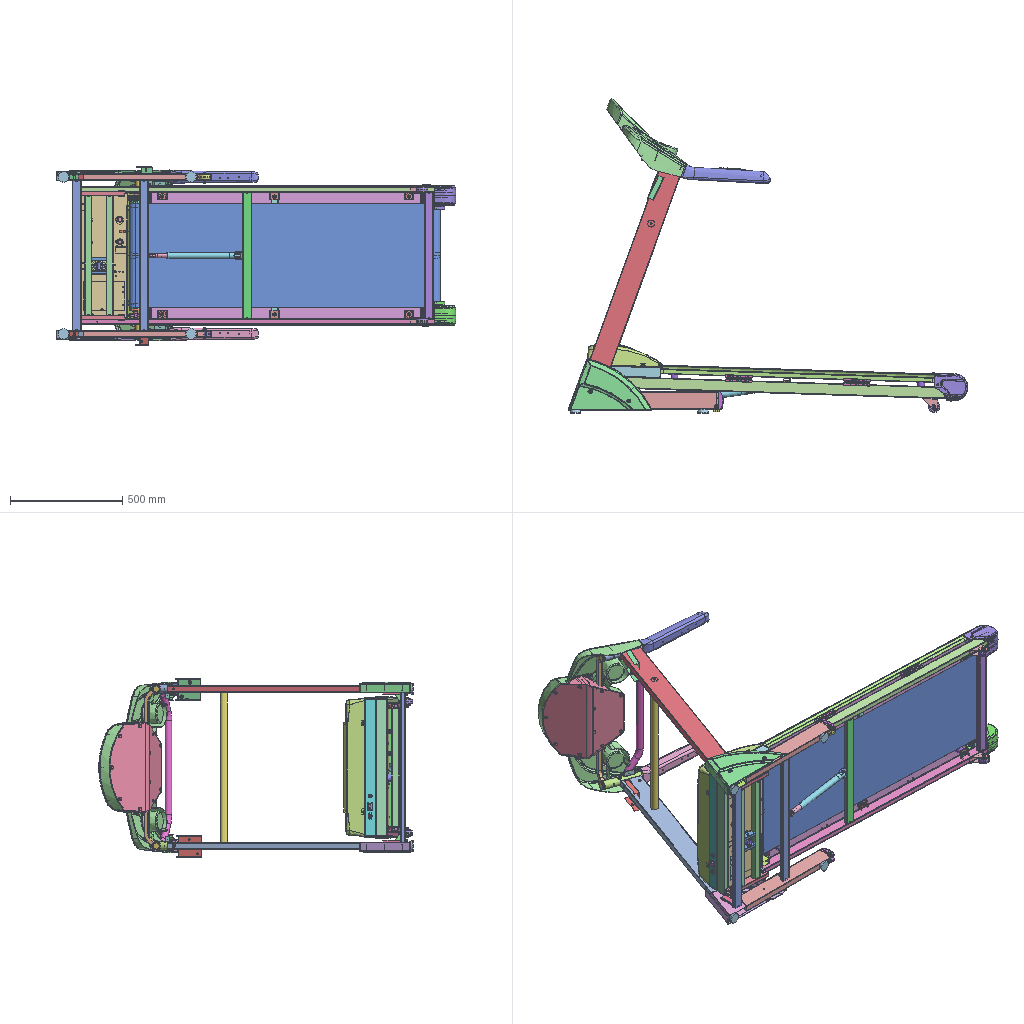Assembly | STEP file | 107 different items | 222 placed | box 1782 x 1401 x 795 mm
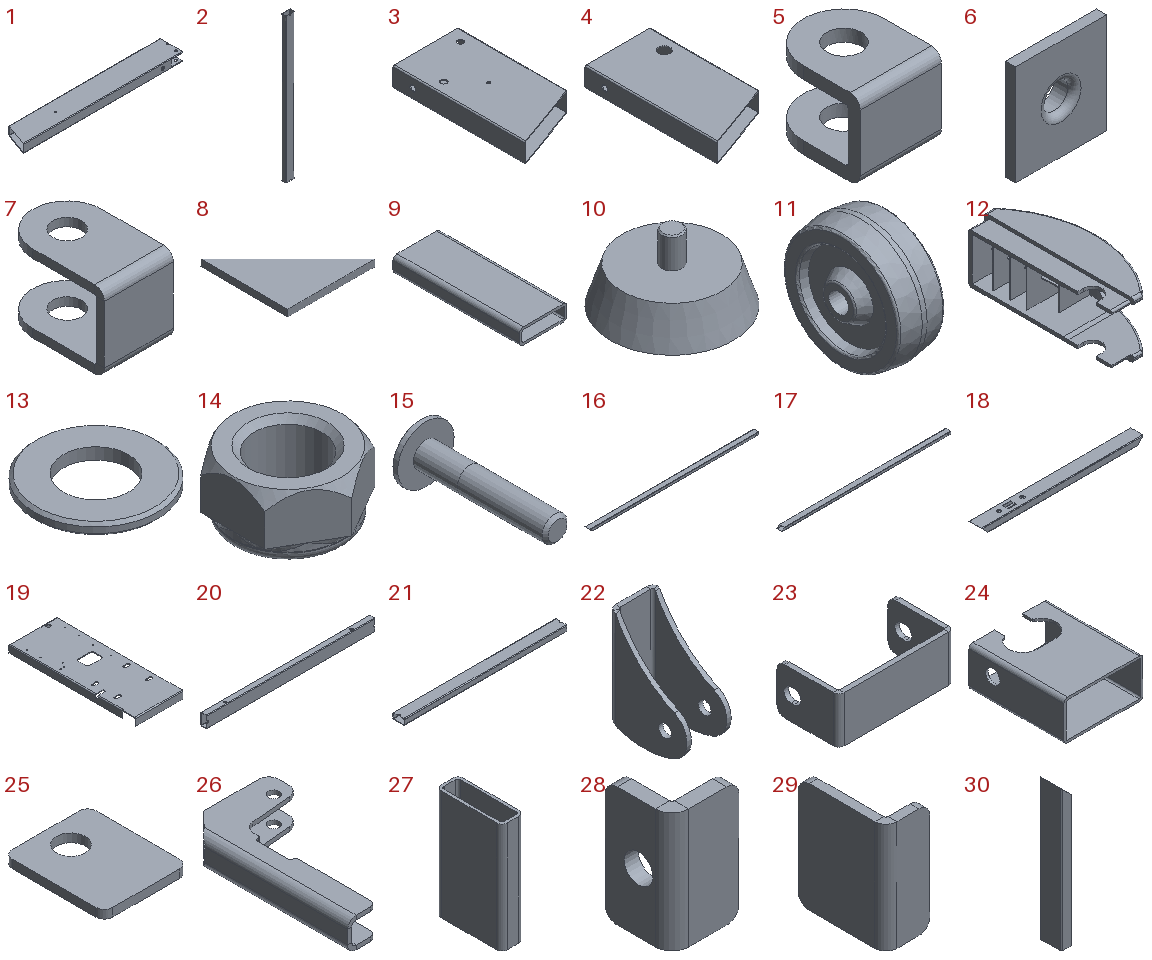Parts list (item | name | quantity | parent item | size | volume):
1 | 7100101 | x2 | in 7100100 | 550 x 80 x 30 mm | 167922 mm3
2 | 7100102 | x2 | in 7100100 | 40 x 20 x 670 mm | 111433 mm3
3 | 7100103L | x1 | in 7100100 | 100 x 200 x 30 mm | 68376 mm3
4 | 7100103R | x1 | in 7100100 | 100 x 200 x 30 mm | 68036 mm3
5 | PN_0011 default | x1 | in 7100100 | 20 x 24 x 19 mm | 3011 mm3
6 | 7100105 | x2 | in 7100100 | 27 x 6 x 30 mm | 2422 mm3
7 | 7100106 | x4 | in 7100100, 7100500 | 25 x 38.5 x 28 mm | 6374 mm3
8 | 7100107 | x4 | in 7100100 | 40 x 40 x 3 mm | 2400 mm3
9 | 7100109 | x2 | in 7100100 | 30 x 80 x 10 mm | 8519 mm3
10 | 7100103W | x4 | in 7100100Z | 48.954 x 48.954 x 27.5 mm | 24706 mm3
11 | PN_0009 variant | x1 | in 7100100Z | 22 x 52.843 x 52.843 mm | 34026 mm3
12 | 7100102W | x2 | in 7100100Z | 30 x 80 x 30 mm | 16145 mm3
13 | PN_0013 variant | x7 | in 7100100Z, 7100500Z | 17 x 17 x 1.6 mm | 252.969 mm3
14 | N208078 | x4 | in 7100100Z, 7100500Z | 13.017 x 15.011 x 7.5 mm | 666.866 mm3
15 | SC40842 variant | x4 | in 7100100Z, 7100500Z | 18 x 46.451 x 18 mm | 2805 mm3
16 | 7100501L | x1 | in 7100500 | 1650 x 50 x 25 mm | 346400 mm3
17 | 7100501R | x1 | in 7100500 | 1650 x 50 x 25 mm | 346388 mm3
18 | 7100502 | x1 | in 7100500 | 613 x 50 x 25 mm | 116984 mm3
19 | PN_0017 default | x1 | in 7100500 | 210 x 564 x 33 mm | 418851 mm3
20 | 7100504 | x1 | in 7100500 | 565 x 20 x 40 mm | 94145 mm3
21 | 7100505 | x1 | in 7100500 | 565 x 40 x 20 mm | 93951 mm3
22 | 7100506 | x2 | in 7100500 | 30 x 53 x 70.522 mm | 17329 mm3
23 | 7100507 | x2 | in 7100500 | 75 x 40 x 30 mm | 12701 mm3
24 | 7100508 | x1 | in 7100500 | 50 x 60 x 25 mm | 11554 mm3
25 | 7100509 | x1 | in 7100500 | 50 x 60 x 5 mm | 13731 mm3
26 | 7100510 | x1 | in 7100500 | 84 x 160 x 29 mm | 53248 mm3
27 | 7100511 | x2 | in 7100500 | 10 x 30 x 50 mm | 4316 mm3
28 | 7100513 | x4 | in 7100500 | 14 x 14 x 25 mm | 1710 mm3
29 | 7100514 | x2 | in 7100500 | 10 x 20 x 25 mm | 1357 mm3
30 | 7100515 | x1 | in 7100500 | 25 x 50 x 325 mm | 66092 mm3
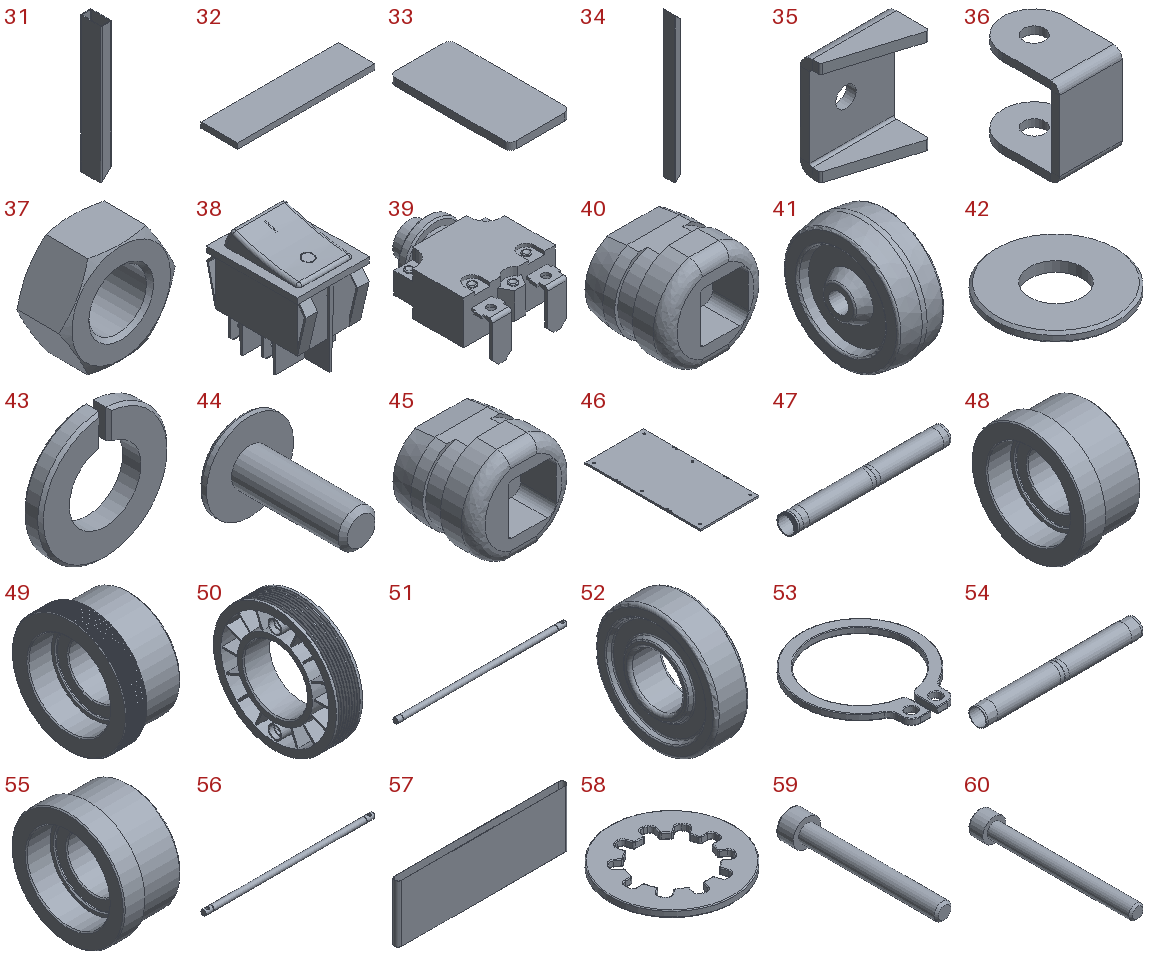31 | 7100516 | x1 | in 7100500 | 25 x 50 x 325 mm | 65710 mm3
32 | 7100517 | x2 | in 7100500 | 75 x 20 x 3 mm | 4500 mm3
33 | 7100518 | x2 | in 7100500 | 25 x 50 x 3 mm | 3734 mm3
34 | 7100519 | x1 | in 7100500 | 25 x 50 x 613 mm | 124358 mm3
35 | 7100520 | x6 | in 7100500 | 35 x 18.649 x 43 mm | 8130 mm3
36 | 7100521 | x1 | in 7100500 | 25 x 35 x 35 mm | 6553 mm3
37 | N108078 | x19 | in 7100500, 7101200, 7100201LZ, 7100201RZ | 16.166 x 7 x 14 mm | 821.972 mm3
38 | EP002 | x1 | in 7100500Z | 25 x 34.5 x 34.784 mm | 14567 mm3
39 | EC002 | x1 | in 7100500Z | 29.3 x 39.3 x 19.65 mm | 10331 mm3
40 | SB6R-3_Default | x1 | in 7100500Z | 17 x 14 x 16 mm | 1519 mm3
41 | PN_0003 variant | x2 | in 7100500Z | 22 x 52.843 x 52.843 mm | 34026 mm3
42 | PN_0019 variant | x6 | in 7100500Z | 9.8 x 9.8 x 0.8 mm | 48.045 mm3
43 | W204009 | x5 | in 7100500Z | 9.2 x 1.3 x 9.193 mm | 57.255 mm3
44 | SD10412 | x8 | in 7100500Z | 9.4 x 14.503 x 9.4 mm | 245.335 mm3
45 | SB5R-2_Default | x1 | in 7100500Z | 17 x 14 x 16 mm | 1519 mm3
46 | DECAK 601 | x1 | in 7100500Z | 605 x 1200 x 18 mm | 13042894 mm3
47 | PN_0012 default | x1 | in 7100700ZA | 495 x 56 x 56 mm | 244128 mm3
48 | PN_0015 default | x1 | in 7100700ZA | 30 x 55.001 x 55.001 mm | 38129 mm3
49 | PN_0014 default | x1 | in 7100700ZA | 30 x 55.999 x 56 mm | 38879 mm3
50 | PN_0002 default | x1 | in 7100700ZA | 23 x 108.001 x 108.001 mm | 96628 mm3
51 | 7100702 | x1 | in 7100700Z | 565 x 17 x 17 mm | 128589 mm3
52 | PL6203ZZA default | x4 | in 7100700Z, 7100800Z | 11 x 40 x 40 mm | 9892 mm3
53 | PN_0018 variant | x4 | in 7100700Z, 7100800Z | 19 x 21.5 x 1 mm | 101.865 mm3
54 | PN_0001 default | x1 | in 7100800ZA | 485 x 56 x 56 mm | 236794 mm3
55 | PN_0016 default | x2 | in 7100800ZA | 30 x 54.43 x 54.43 mm | 37639 mm3
56 | 7100803 | x1 | in 7100800Z | 560 x 17 x 17 mm | 125657 mm3
57 | RUBE 601 | x1 | in 7100500Z | 1389 x 59.2 x 465 mm | 2113671 mm3
58 | PN_0008 variant | x3 | in 7100500Z | 15 x 15 x 0.8 mm | 82.689 mm3
59 | SA10865 | x1 | in 7100500Z | 13 x 73 x 13 mm | 4160 mm3
60 | SA10880 | x2 | in 7100500Z | 13 x 88 x 13 mm | 4914 mm3
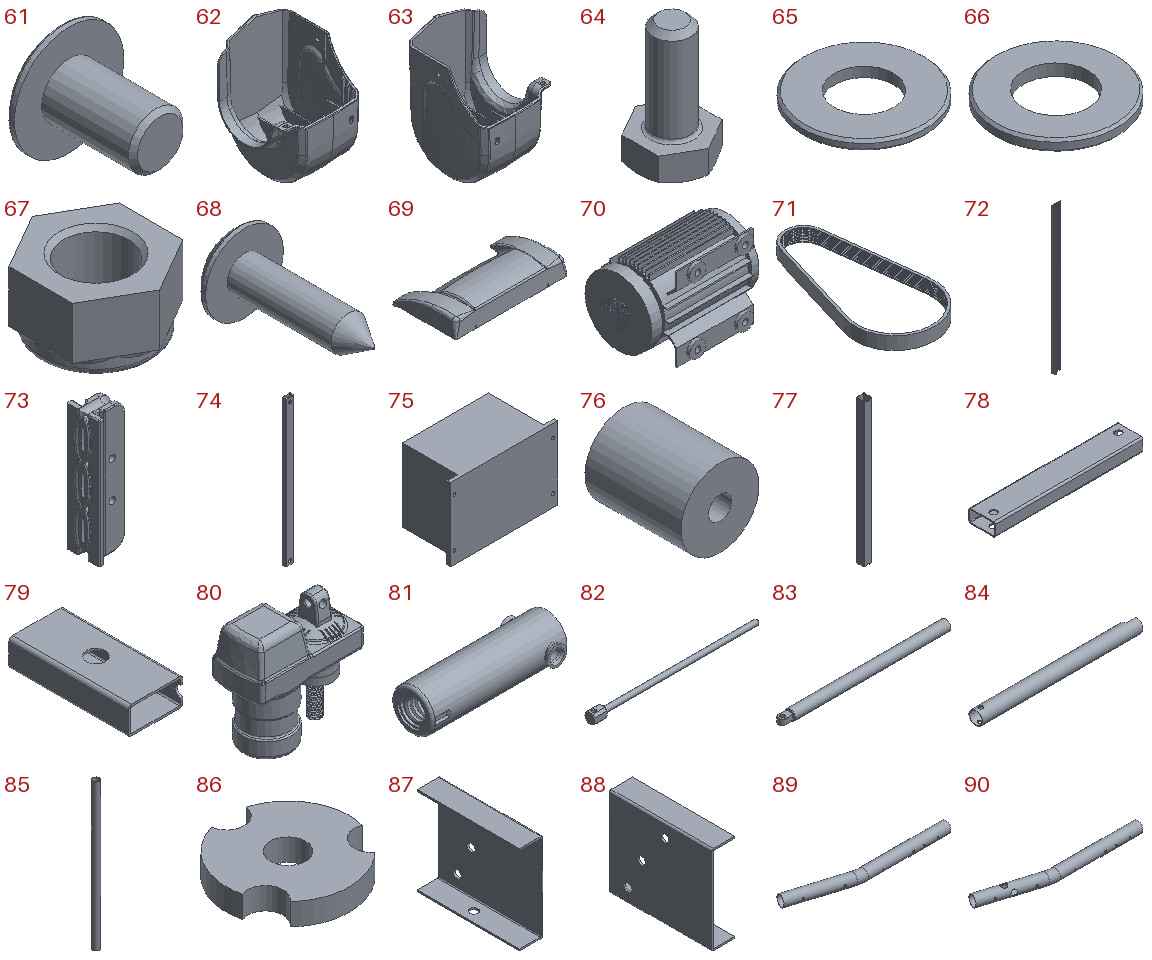61 | SD10610 | x3 | in 7100500Z | 12 x 12.964 x 12 mm | 479.053 mm3
62 | EDN CAP 601L | x1 | in 7100500Z | - | 183620 mm3
63 | EDN CAP 601R | x1 | in 7100500Z | - | 183322 mm3
64 | SI1025_M10 | x4 | in 7100500Z | 17 x 19.6 x 32 mm | 3678 mm3
65 | PN_0005 variant | x4 | in 7100500Z | 25 x 25 x 2 mm | 736.18 mm3
66 | PN_0004 variant | x4 | in 7100500Z | 21 x 21 x 2 mm | 492.233 mm3
67 | N210095 | x4 | in 7100500Z | 17 x 19.63 x 10.5 mm | 1722 mm3
68 | SD20415 | x2 | in 7100500Z | 9 x 17.646 x 9 mm | 255.973 mm3
69 | 96L | x1 | in 7100500Z | - | -
70 | AC MOTOR 1.5KW | x1 | in 7100500Z | 263.5 x 156.005 x 174 mm | 3095920 mm3
71 | DE200JS8 | x1 | in 7100500Z | 111 x 221.3 x 18 mm | 22925 mm3
72 | SIDE | x2 | in 7100500Z | 76 x 36.5 x 1228 mm | 489204 mm3
73 | jianzhendian | x2 | in 7100500Z | 30 x 30 x 117 mm | 56101 mm3
74 | 7100901 | x1 | in 7100500Z | 30 x 15 x 555 mm | 54621 mm3
75 | frequency converter | x1 | in 7100500Z | 185 x 101 x 126 mm | 1922919 mm3
76 | DECH02 | x4 | in 7100500Z | 30 x 37 x 30 mm | 23800 mm3
77 | PN_0007 default | x2 | in 7100400 | 30 x 30 x 532 mm | 88457 mm3
78 | 7100402 | x2 | in 7100400 | 225 x 40 x 20 mm | 36971 mm3
79 | 7100403 | x2 | in 7100400 | 30 x 65 x 15 mm | 6216 mm3
80 | PN_0006 default | x1 | in 710 | 148.1 x 70.5 x 151.812 mm | 777031 mm3
81 | J09 601B | x1 | in 710 | 115 x 41.999 x 35 mm | 49295 mm3
82 | GAS SHOCK 609S | x1 | in 710 | 353.5 x 20 x 20 mm | 34694 mm3
83 | GAS SHOCK 609X | x1 | in 710 | 359 x 22 x 22 mm | 94119 mm3
84 | GAS SHOCK 610W | x1 | in 710 | 330 x 28 x 28 mm | 39789 mm3
85 | 7101301 | x1 | in 7101300 | 31.8 x 31.8 x 725 mm | 103519 mm3
86 | PN_0010 default | x2 | in 7101300 | 28 x 27.429 x 5 mm | 2473 mm3
87 | 7100108L | x2 | in 7101200, 7100201LZ | 25 x 110 x 95 mm | 29808 mm3
88 | 7100108R | x2 | in 7101200, 7100201RZ | 25 x 110 x 95 mm | 29808 mm3
89 | 7101202L | x1 | in 7101200 | 530.631 x 103.035 x 38.1 mm | 88866 mm3
90 | 7101202R | x1 | in 7101200 | 530.631 x 103.035 x 38.1 mm | 88372 mm3
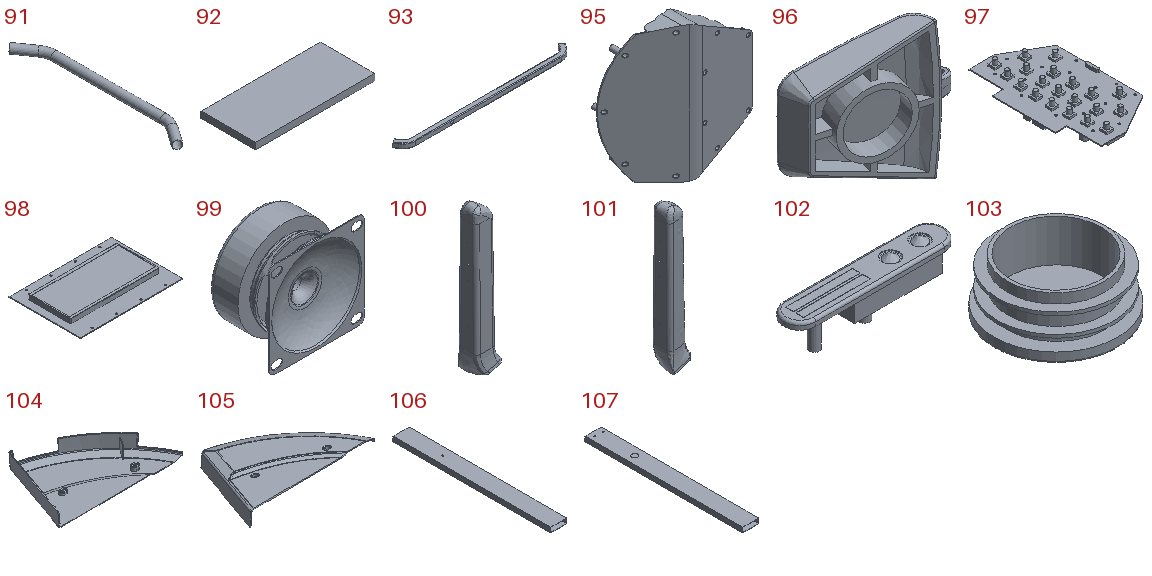91 | 7101203 | x1 | in 7101200 | 89.278 x 660.628 x 31.8 mm | 96707 mm3
92 | 7101204 | x2 | in 7101200 | 55 x 25 x 3 mm | 4125 mm3
93 | 7101205 | x1 | in 7101200 | 697.147 x 49.49 x 20 mm | 75230 mm3
94 | NA609S-A | x1 | in NA609SZ | - | -
95 | NA609S-B | x1 | in NA609SZ | 340.609 x 142.904 x 405.431 mm | 455741 mm3
96 | NA609S-C | x1 | in NA609SZ | 35.148 x 15.37 x 38.312 mm | 3411 mm3
97 | PCB Plate-618 | x1 | in NA609SZ | 132 x 230 x 23.4 mm | 58668 mm3
98 | - | x1 | in NA609SZ | 210 x 145 x 11 mm | 188408 mm3
99 | - | x2 | in NA609SZ | 50 x 31.5 x 50 mm | 33375 mm3
100 | 7101206LW | x1 | in 7101200Z | 71.872 x 63.257 x 397.874 mm | 548309 mm3
101 | 7101206RW | x1 | in 7101200Z | 71.871 x 63.257 x 397.874 mm | 548109 mm3
102 | 7101207W | x2 | in 7101200Z | 119.5 x 24 x 32.509 mm | 28513 mm3
103 | 7101208W | x2 | in 7101200Z | 38 x 38 x 16 mm | 5202 mm3
104 | right column cover | x1 | in 710 | 372.789 x 229.022 x 48 mm | 179177 mm3
105 | left column cover | x1 | in 710 | 372.789 x 229.022 x 48 mm | 179176 mm3
106 | 7100201L | x1 | in 7100201LZ | 100 x 950 x 30 mm | 355925 mm3
107 | 7100201R | x1 | in 7100201RZ | 100 x 950 x 30 mm | 355925 mm3
Placements (level | parent | child | x y z in mm | rotation matrix by rows):
1 | 710 | 7100100Z | 319.734 -99.186 350.0 | 1 0 0 0 1 0 0 0 1
2 | 7100100Z | 7100100 | -0.0 -0.0 -0.0 | 1 0 0 0 1 0 0 0 1
3 | 7100100 | 7100101 | -0.0 -0.0 -0.0 | 1 0 0 0 1 0 0 0 1
3 | 7100100 | 7100101 | -0.0 -0.0 -700.0 | 1 0 0 0 1 0 0 0 1
3 | 7100100 | 7100102 | -280.0 20.0 -350.0 | 1 0 0 0 1 0 0 0 1
3 | 7100100 | 7100102 | -580.0 20.0 -350.0 | 1 0 0 0 1 0 0 0 1
3 | 7100100 | 7100103L | -609.433 -17.101 -0.0 | 0.9397 0.342 0 -0.342 0.9397 0 0 0 1
3 | 7100100 | 7100103R | -609.433 -17.101 -700.0 | 0.9397 0.342 0 -0.342 0.9397 0 0 0 1
3 | 7100100 | PN_0011 default | -260.0 30.0 -350.0 | 0 1 0 -1 0 0 0 0 1
3 | 7100100 | 7100105 | -638.73 0.0 0.0 | 0 0 -1 0 1 0 1 0 -0
3 | 7100100 | 7100105 | -638.73 0.0 -700.0 | 0 0 1 0 1 0 -1 0 0
3 | 7100100 | 7100106 | -580.0 40.0 -74.0 | 1 0 0 0 1 0 0 0 1
3 | 7100100 | 7100106 | -580.0 40.0 -626.0 | 1 0 0 0 1 0 0 0 1
3 | 7100100 | 7100107 | -560.0 80.0 -685.0 | 0 0 -1 0 1 0 1 0 0
3 | 7100100 | 7100107 | -563.0 80.0 -15.0 | 0 0 1 0 1 0 -1 0 0
3 | 7100100 | 7100107 | -281.5 80.0 -15.0 | 0 0 1 0 1 0 -1 0 0
3 | 7100100 | 7100107 | -281.5 40.0 -645.0 | 0 0 1 1 0 0 0 1 -0
3 | 7100100 | 7100109 | -599.674 40.0 -672.775 | 1 0 0 0 1 0 0 0 1
3 | 7100100 | 7100109 | -599.674 40.0 -12.775 | 1 0 0 0 1 0 0 0 1
2 | 7100100Z | 7100103W | -638.73 0.0 -0.0 | 0.9991 -0.04147 0 0 0 1 -0.04147 -0.9991 0
2 | 7100100Z | 7100103W | -70.0 -0.0 0.0 | -0.9344 0.3562 0 0 0 1 0.3562 0.9344 0
2 | 7100100Z | PN_0009 variant | -10.0 15.0 -0.0 | 0 0 1 0 1 0 -1 0 0
2 | 7100100Z | 7100102W | -0.0 40.0 -0.0 | 1 0 0 0 1 0 0 0 1
2 | 7100100Z | PN_0013 variant | -10.0 15.0 -16.6 | 1 0 0 0 1 0 0 0 1
2 | 7100100Z | PN_0013 variant | -10.0 15.0 -683.4 | -0.9237 -0.383 0 -0.383 0.9237 0 0 0 -1
2 | 7100100Z | N208078 | -10.0 15.0 -22.1 | 1 0 0 0 1 0 0 0 1
2 | 7100100Z | N208078 | -10.0 15.0 -677.9 | -0.9237 -0.383 0 -0.383 0.9237 0 0 0 -1
2 | 7100100Z | SC40842 variant | -10.0 15.0 15.0 | 1 0 0 0 0 -1 0 1 0
2 | 7100100Z | SC40842 variant | -10.0 15.0 -715.0 | 1 0 0 0 0 1 0 -1 0
2 | 7100100Z | 7100103W | -638.73 0.0 -700.0 | 0.9991 -0.04147 0 0 0 1 -0.04147 -0.9991 0
2 | 7100100Z | 7100103W | -70.0 -0.0 -700.0 | -0.9344 0.3562 0 0 0 1 0.3562 0.9344 0
2 | 7100100Z | 7100102W | -0.0 40.0 -700.0 | 1 0 0 0 1 0 0 0 1
1 | 710 | 7100500Z | 446.175 68.129 310.459 | 0.9995 0.03221 0 -0.03221 0.9995 0 0 0 1
2 | 7100500Z | 7100500 | -0.0 -0.0 -0.0 | 1 0 0 0 1 0 0 0 1
3 | 7100500 | 7100501L | 112.255 -64.436 -15.459 | 1 0 0 0 1 0 0 0 1
3 | 7100500 | 7100501R | 112.255 -64.436 -605.459 | 1 0 0 0 1 0 0 0 1
3 | 7100500 | 7100502 | -700.245 -14.436 -310.459 | 0 0 -1 0 1 0 1 0 0
3 | 7100500 | PN_0017 default | -687.745 -86.436 -310.459 | -1 0 0 0 0 -1 0 -1 0
3 | 7100500 | 7100504 | 867.255 -79.436 -310.459 | 0 0 1 0 1 0 -1 0 -0
3 | 7100500 | 7100505 | 57.255 -79.436 -310.459 | 0 -1 0 0 0 -1 1 0 0
3 | 7100500 | 7100506 | 825.755 -89.436 -17.959 | 0 0 -1 0 1 0 1 0 0
3 | 7100500 | 7100506 | 825.755 -89.436 -602.959 | 0 0 -1 0 1 0 1 0 0
3 | 7100500 | 7100507 | 899.755 -24.436 -32.959 | 1 0 0 0 0 1 0 -1 0
3 | 7100500 | 7100507 | 899.755 -24.436 -587.959 | 1 0 0 0 0 -1 0 1 -0
3 | 7100500 | 7100508 | -442.745 -39.436 -580.459 | 1 0 0 0 1 0 0 0 1
3 | 7100500 | 7100509 | -442.745 -69.436 -32.959 | 1 0 0 0 1 0 0 0 1
3 | 7100500 | 7100510 | -666.745 73.564 -357.459 | 1 0 0 0 1 0 0 0 1
3 | 7100500 | 7100511 | -505.745 -137.337 -301.977 | 0 0 1 -1 0 0 0 -1 0
3 | 7100500 | 7100511 | -662.745 -25.535 -109.977 | 0 0 -1 1 0 0 0 -1 -0
3 | 7100500 | 7100513 | -465.745 10.564 -614.959 | 0 0 -1 0 1 0 1 0 0
3 | 7100500 | 7100513 | -712.745 10.564 -112.959 | 1 0 0 0 1 0 0 0 1
3 | 7100500 | 7100513 | -465.745 10.564 -5.959 | 0 0 1 0 1 0 -1 0 0
3 | 7100500 | 7100513 | -712.745 10.564 -507.959 | 1 0 0 0 1 0 0 0 1
3 | 7100500 | 7100514 | 849.755 -39.436 -2.959 | 0 0 1 0 1 0 -1 0 -0
3 | 7100500 | 7100514 | 849.755 -39.436 -617.959 | 0 0 -1 0 1 0 1 0 0
3 | 7100500 | 7100515 | -387.745 -14.436 -605.459 | 0 0 -1 0 1 0 1 0 0
3 | 7100500 | 7100516 | -712.745 -14.436 -15.459 | 0 0 1 0 1 0 -1 0 -0
3 | 7100500 | 7100517 | 899.755 -42.436 -37.959 | 1 0 0 0 0 1 0 -1 -0
3 | 7100500 | 7100517 | 899.755 -42.436 -582.959 | 1 0 0 0 0 1 0 -1 0
3 | 7100500 | 7100518 | -384.745 -14.436 -15.459 | 0 0 -1 0 1 0 1 0 0
3 | 7100500 | 7100518 | -387.745 -14.436 -605.459 | 0 0 1 0 1 0 -1 0 -0
3 | 7100500 | 7100519 | -700.245 -64.436 -616.959 | 1 0 0 0 1 0 0 0 1
3 | 7100500 | 7100520 | -322.745 -56.436 -27.959 | 0 0 -1 0 1 0 1 0 0
3 | 7100500 | 7100520 | 777.255 -56.436 -27.959 | 0 0 -1 0 1 0 1 0 0
3 | 7100500 | 7100520 | -322.745 -56.436 -592.959 | 0 0 1 0 1 0 -1 0 -0
3 | 7100500 | 7100520 | 777.255 -56.436 -592.959 | 0 0 1 0 1 0 -1 0 -0
3 | 7100500 | 7100520 | 177.255 -36.436 -592.959 | 0 0 1 0 1 0 -1 0 -0
3 | 7100500 | 7100520 | 177.255 -36.436 -27.959 | 0 0 -1 0 1 0 1 0 -0
3 | 7100500 | 7100521 | 37.255 -81.936 -310.459 | 0 -1 0 1 0 0 0 0 1
3 | 7100500 | 7100106 | -502.745 -89.436 -586.459 | 1 0 0 0 -1 0 0 0 -1
3 | 7100500 | 7100106 | -502.745 -89.436 -34.459 | 1 0 0 0 -1 0 0 0 -1
3 | 7100500 | N108078 | -484.245 -80.436 -203.459 | 0 -1 0 0.866 0 -0.5 0.5 0 0.866
3 | 7100500 | N108078 | -322.745 -63.936 -47.959 | 0.866 0 -0.5 0 1 0 0.5 0 0.866
3 | 7100500 | N108078 | -322.745 -63.936 -572.959 | 0.866 0 -0.5 0 1 0 0.5 0 0.866
3 | 7100500 | N108078 | 177.255 -43.936 -47.959 | 0.866 0 -0.5 0 1 0 0.5 0 0.866
3 | 7100500 | N108078 | 777.255 -63.936 -47.959 | 0.866 0 -0.5 0 1 0 0.5 0 0.866
3 | 7100500 | N108078 | 777.255 -63.936 -572.959 | 0.8429 0 -0.5381 0 1 0 0.5381 0 0.8429
3 | 7100500 | N108078 | 177.255 -43.936 -572.959 | 0.866 0 -0.5 0 1 0 0.5 0 0.866
2 | 7100500Z | EP002 | -712.745 -14.186 -485.709 | 0 0 -1 -1 0 0 0 1 0
2 | 7100500Z | EC002 | -655.465 -21.336 -484.294 | 0 -1 0 0 0 -1 1 0 0
2 | 7100500Z | SB6R-3_Default | -718.245 -14.524 -437.359 | 0 1 0 -1 0 0 0 0 1
2 | 7100500Z | PN_0003 variant | 837.255 -127.436 -16.959 | 0 0.005777 -1 0 1 0.005777 1 0 0
2 | 7100500Z | PN_0003 variant | 837.255 -127.436 -601.959 | 0 0.01299 0.9999 0 0.9999 -0.01299 -1 0 0
2 | 7100500Z | PN_0019 variant | -497.745 -82.636 -532.459 | 1 0 0 0 0 -1 0 1 -0
2 | 7100500Z | PN_0019 variant | -590.745 -84.436 -552.459 | 1 0 0 0 0 1 0 -1 0
2 | 7100500Z | PN_0019 variant | -662.745 -86.436 -322.459 | 0.9885 -0.1514 0 0 0 1 -0.1514 -0.9885 0
2 | 7100500Z | PN_0019 variant | -532.745 -86.436 -382.459 | 1 0 0 0 0 1 0 -1 0
2 | 7100500Z | PN_0019 variant | -667.745 -84.436 -532.459 | 0.8986 -0.4389 0 0 0 1 -0.4389 -0.8986 0
2 | 7100500Z | W204009 | -497.745 -82.636 -532.459 | -0.2314 0 0.9729 0 1 0 -0.9729 0 -0.2314
2 | 7100500Z | W204009 | -662.745 -84.336 -322.459 | 0.9816 0 -0.1911 0 -1 0 -0.1911 0 -0.9816
2 | 7100500Z | W204009 | -532.745 -84.336 -382.459 | 1 0 0 0 -1 0 0 0 -1
2 | 7100500Z | W204009 | -667.745 -82.336 -532.459 | 1 0 0 0 -1 0 0 0 -1
2 | 7100500Z | SD10412 | -532.745 -84.336 -382.459 | -0.8802 0 -0.4746 0 1 0 0.4746 0 -0.8802
2 | 7100500Z | SD10412 | -662.745 -84.336 -322.459 | 0.9884 0 0.152 0 1 0 -0.152 0 0.9884
2 | 7100500Z | SD10412 | -497.745 -81.336 -532.459 | 0.8688 0 -0.4951 0 1 0 0.4951 0 0.8688
2 | 7100500Z | SD10412 | -532.745 -81.336 -352.459 | -0.4579 0 -0.889 0 1 0 0.889 0 -0.4579
2 | 7100500Z | PN_0019 variant | -532.745 -83.436 -352.459 | 1 0 0 0 0 1 0 -1 0
2 | 7100500Z | W204009 | -532.745 -81.336 -352.459 | 1 0 0 0 -1 0 0 0 -1
2 | 7100500Z | PN_0013 variant | 837.255 -127.436 -34.559 | 1 0 0 0 1 0 0 0 1
2 | 7100500Z | PN_0013 variant | 837.255 -127.436 -586.359 | -1 0 0 0 1 0 0 0 -1
2 | 7100500Z | SC40842 variant | 837.255 -127.436 -1.959 | 1 0 0 0 0 -1 0 1 -0
2 | 7100500Z | SC40842 variant | 837.255 -127.436 -618.959 | 1 0 0 0 0 1 0 -1 -0
2 | 7100500Z | N208078 | 837.255 -127.436 -40.059 | 1 0 0 0 1 0 0 0 1
2 | 7100500Z | N208078 | 837.255 -127.436 -580.859 | -0.8858 -0.464 0 -0.464 0.8858 0 0 0 -1
2 | 7100500Z | SB5R-2_Default | -637.579 -94.936 -577.464 | -0.9995 0 -0.03043 0 1 0 0.03043 0 -0.9995
2 | 7100500Z | DECAK 601 | 227.255 -10.436 -310.459 | 0 -1 0 0 0 1 -1 0 0
2 | 7100500Z | 7100700Z | -442.745 -24.436 -299.659 | 0 1 0 0 0 -1 -1 0 -0
3 | 7100700Z | 7100700ZA | 0.0 0.0 -0.0 | 1 0 0 0 1 0 0 0 1
4 | 7100700ZA | PN_0012 default | -0.0 -0.0 -0.0 | 1 0 0 0 1 0 0 0 1
4 | 7100700ZA | PN_0015 default | 257.5 -0.0 0.0 | -1 0 0 0 0.5057 -0.8627 0 -0.8627 -0.5057
4 | 7100700ZA | PN_0014 default | -257.5 -0.0 0.0 | 1 0 0 0 1 0 0 0 1
4 | 7100700ZA | PN_0002 default | -257.5 -0.0 0.0 | 1 0 0 0 1 0 0 0 1
3 | 7100700Z | 7100702 | -1.7 0.0 -0.0 | 1 0 0 0 0 1 0 -1 -0
3 | 7100700Z | PL6203ZZA default | 246.5 8.5 -0.0 | 1 0 0 0 1 0 0 0 1
3 | 7100700Z | PL6203ZZA default | -257.5 8.5 -0.0 | 1 0 0 0 1 0 0 0 1
3 | 7100700Z | PN_0018 variant | 257.6 0.0 -0.0 | 0 0 1 0 1 0 -1 0 -0
3 | 7100700Z | PN_0018 variant | -258.6 0.0 -0.0 | 0 0 1 0 1 0 -1 0 -0
2 | 7100500Z | 7100800Z | 887.255 -24.436 -309.459 | 0 0 -1 0 1 0 1 0 0
3 | 7100800Z | 7100800ZA | 0.0 0.0 0.0 | 1 0 0 0 1 0 0 0 1
4 | 7100800ZA | PN_0001 default | -0.0 -0.0 -0.0 | 1 0 0 0 1 0 0 0 1
4 | 7100800ZA | PN_0016 default | -252.5 -0.0 0.0 | 1 0 0 0 1 0 0 0 1
4 | 7100800ZA | PN_0016 default | 252.5 0.0 -0.0 | -1 0 0 0 0.3818 -0.9242 0 -0.9242 -0.3818
3 | 7100800Z | PL6203ZZA default | -252.5 8.5 -0.0 | 1 0 0 0 1 0 0 0 1
3 | 7100800Z | PL6203ZZA default | 241.5 8.5 -0.0 | 1 0 0 0 1 0 0 0 1
3 | 7100800Z | PN_0018 variant | 252.6 0.0 0.0 | 0 0 1 0 1 0 -1 0 0
3 | 7100800Z | PN_0018 variant | -252.8 -0.0 0.0 | 0 0 -1 0 1 0 1 0 0
3 | 7100800Z | 7100803 | 0.0 0.0 0.0 | 1 0 0 0 1 0 0 0 1
2 | 7100500Z | RUBE 601 | 805.755 -24.436 -310.459 | 1 0 0 0 1 0 0 0 1
2 | 7100500Z | PN_0008 variant | 938.055 -24.436 -41.959 | 0 0 -1 0 1 0 1 0 -0
2 | 7100500Z | PN_0008 variant | -468.545 -24.436 -577.959 | 0 0 1 0 1 0 -1 0 0
2 | 7100500Z | PN_0013 variant | 939.655 -24.436 -41.959 | 0 0 -1 0 1 0 1 0 -0
2 | 7100500Z | PN_0013 variant | -470.145 -24.436 -577.959 | 0 0 1 0 1 0 -1 0 0
2 | 7100500Z | SA10865 | -470.145 -24.436 -577.959 | 0 -1 0 1 0 0 0 0 1
2 | 7100500Z | SA10880 | 939.655 -24.436 -41.959 | 0 1 0 -0.891 0 0.4541 0.4541 0 0.891
2 | 7100500Z | SD10412 | 890.255 -81.436 -97.959 | 0 1 0 -1 0 0 0 0 1
2 | 7100500Z | SD10412 | 890.255 -81.436 -522.959 | 0 1 0 -1 0 0 0 0 1
2 | 7100500Z | SD10610 | -465.745 17.564 -2.959 | 0.9957 0 -0.09225 -0.09225 0 -0.9957 0 1 0
2 | 7100500Z | SD10610 | -715.745 17.564 -112.959 | 0 -1 0 1 0 0 0 0 1
2 | 7100500Z | SD10610 | -465.745 17.564 -617.959 | -0.9199 0 0.3922 -0.3922 0 -0.9199 0 -1 -0
2 | 7100500Z | EDN CAP 601L | 824.255 20.504 -42.468 | 0 0 -1 0 1 0 1 0 -0
2 | 7100500Z | EDN CAP 601R | 824.255 20.504 -578.45 | 0 0 -1 0 1 0 1 0 -0
2 | 7100500Z | PN_0008 variant | 938.055 -24.436 -576.959 | 0 0 -1 0 1 0 1 0 -0
2 | 7100500Z | PN_0013 variant | 939.655 -24.436 -576.959 | 0 0 -1 0 1 0 1 0 -0
2 | 7100500Z | SA10880 | 939.655 -24.436 -576.959 | 0 1 0 -0.891 0 0.4541 0.4541 0 0.891
2 | 7100500Z | SI1025_M10 | -650.245 -96.436 -149.459 | 0.7133 -0.7008 0 0 0 1 -0.7008 -0.7133 -0
2 | 7100500Z | SI1025_M10 | -650.245 -96.436 -249.459 | -0.1244 0.9922 0 0 0 1 0.9922 0.1244 -0
2 | 7100500Z | SI1025_M10 | -510.245 -96.436 -149.459 | 0.87 -0.493 0 0 0 1 -0.493 -0.87 -0
2 | 7100500Z | SI1025_M10 | -510.245 -96.436 -249.459 | 0.4078 -0.9131 0 0 0 1 -0.9131 -0.4078 0
2 | 7100500Z | PN_0005 variant | -510.245 -84.436 -249.459 | 1 0 0 0 0 -1 0 1 0
2 | 7100500Z | PN_0005 variant | -510.245 -84.436 -149.459 | 1 0 0 0 0 -1 0 1 0
2 | 7100500Z | PN_0005 variant | -650.245 -84.436 -249.459 | 1 0 0 0 0 -1 0 1 0
2 | 7100500Z | PN_0005 variant | -650.245 -84.436 -149.459 | 1 0 0 0 0 -1 0 1 0
2 | 7100500Z | PN_0004 variant | -650.245 -79.436 -149.459 | 1 0 0 0 0 -1 0 1 0
2 | 7100500Z | PN_0004 variant | -510.245 -79.436 -249.459 | 1 0 0 0 0 -1 0 1 0
2 | 7100500Z | PN_0004 variant | -510.245 -79.436 -149.459 | 1 0 0 0 0 -1 0 1 0
2 | 7100500Z | PN_0004 variant | -650.245 -79.436 -249.459 | 0.697 0.7171 0 0 0 -1 -0.7171 0.697 0
2 | 7100500Z | N210095 | -650.245 -71.436 -149.459 | 1 0 0 0 0 -1 0 1 0
2 | 7100500Z | N210095 | -650.245 -71.436 -249.459 | 1 0 0 0 0 -1 0 1 0
2 | 7100500Z | N210095 | -510.245 -71.436 -149.459 | 1 0 0 0 0 -1 0 1 0
2 | 7100500Z | N210095 | -510.245 -71.436 -249.459 | 1 0 0 0 0 -1 0 1 0
2 | 7100500Z | SD10412 | 912.255 -96.742 -15.459 | 0.3726 0 -0.928 0 -1 0 -0.928 0 -0.3726
2 | 7100500Z | SD10412 | 912.255 -96.742 -605.459 | -0.0932 0 -0.9956 0 -1 0 -0.9956 0 0.0932
2 | 7100500Z | SD20415 | 851.255 -29.496 4.041 | 1 0 0 0 0 -1 0 1 -0
2 | 7100500Z | SD20415 | 851.255 -29.496 -624.959 | 1 0 0 0 0 1 0 -1 -0
2 | 7100500Z | 96L | -545.552 5.354 -310.459 | 0 1 0 0 0 1 1 0 -0
2 | 7100500Z | AC MOTOR 1.5KW | -581.276 -5.436 -40.435 | 0 0 1 0 1 0 -1 0 0
2 | 7100500Z | DE200JS8 | -147.941 454.58 -53.659 | 0.04941 -0.9988 0 0.9988 0.04941 0 0 0 1
2 | 7100500Z | SIDE | 843.255 17.564 0.0413 | 0 0 1 0 1 0 -1 0 0
2 | 7100500Z | SIDE | -384.745 17.564 -620.959 | 0 0 -1 0 1 0 1 0 -0
2 | 7100500Z | jianzhendian | -94.245 -30.366 -13.959 | 0 0 1 0 1 0 -1 0 -0
2 | 7100500Z | jianzhendian | 431.755 -30.366 -13.959 | 0 0 1 0 1 0 -1 0 -0
2 | 7100500Z | 7100901 | 177.255 -26.936 -311.959 | 1 0 0 0 1 0 0 0 1
2 | 7100500Z | frequency converter | -564.657 -86.436 -520.108 | 1 0 0 0 1 0 0 0 1
2 | 7100500Z | DECH02 | -322.745 -56.436 -572.959 | 1 0 0 0 1 0 0 0 1
2 | 7100500Z | DECH02 | 777.255 -56.436 -572.959 | 1 0 0 0 1 0 0 0 1
2 | 7100500Z | DECH02 | -322.745 -56.436 -47.959 | 1 0 0 0 1 0 0 0 1
2 | 7100500Z | DECH02 | 777.255 -56.436 -47.959 | 1 0 0 0 1 0 0 0 1
1 | 710 | 7100400 | -112.88 -38.983 -0.0 | 0.9992 0.0393 0 -0.0393 0.9992 0 0 0 1
2 | 7100400 | PN_0007 default | -0.0 -0.0 -0.0 | 1 0 0 0 1 0 0 0 1
2 | 7100400 | PN_0007 default | -95.0 0.0 -0.0 | 1 0 0 0 1 0 0 0 1
2 | 7100400 | 7100402 | -160.0 5.0 276.0 | 1 0 0 0 1 0 0 0 1
2 | 7100400 | 7100402 | -160.0 5.0 -276.0 | 1 0 0 0 1 0 0 0 1
2 | 7100400 | 7100403 | -47.5 0.0 -16.5 | 0 1 0 1 0 0 0 0 -1
2 | 7100400 | 7100403 | -47.5 0.0 -76.5 | 0 -1 0 1 0 0 0 0 1
1 | 710 | PN_0006 default | -167.112 81.691 -46.75 | -0.9984 0 -0.05688 -0.05688 0 0.9984 0 1 -0
1 | 710 | J09 601B | -166.202 65.717 -46.75 | 0.05688 0 -0.9984 -0.9984 0 -0.05688 0 1 0
1 | 710 | GAS SHOCK 609S | 438.484 -17.068 -0.0 | -0.9899 0.1414 0 -0.1414 -0.9899 0 0 0 1
1 | 710 | GAS SHOCK 609X | 267.269 -41.532 0.0 | 0.9899 -0.1414 0 0.1414 0.9899 0 0 0 1
1 | 710 | GAS SHOCK 610W | 468.183 -12.825 -0.0 | -0.9899 -0.1414 0 -0.1414 0.9899 0 0 0 -1
1 | 710 | 7101300 | 19.018 726.679 1.0 | 0.03536 0.9994 0 -0.9994 0.03536 0 0 0 1
2 | 7101300 | 7101301 | -2.788 -0.8012 -0.0 | 1 0 0 0 1 0 0 0 1
2 | 7101300 | PN_0010 default | -2.788 -0.8012 352.5 | -0.8814 -0.4723 0 0.4723 -0.8814 0 0 0 1
2 | 7101300 | PN_0010 default | -2.788 -0.8012 -357.5 | -0.8814 -0.4723 0 0.4723 -0.8814 0 0 0 1
1 | 710 | 7101200Z | 247.775 997.523 -27.882 | 0 -0.02963 0.9996 0 0.9996 0.02963 -1 0 -0
2 | 7101200Z | 7101200 | 304.618 225.035 478.871 | 1 0 0 0 1 0 0 0 1
3 | 7101200 | 7100108L | -682.5 -389.81 -688.408 | 0 0 -1 -0.4545 0.8907 0 0.8907 0.4545 -0
3 | 7101200 | 7100108R | 17.5 -278.485 -685.966 | 0 0 -1 0.3697 -0.9291 0 -0.9291 -0.3697 -0
3 | 7101200 | 7101202L | -682.5 -292.615 -224.121 | 0 0 -1 -0.0819 0.9966 0 0.9966 0.0819 -0
3 | 7101200 | 7101202R | 17.5 -292.615 -224.121 | 0 0 -1 -0.0819 0.9966 0 0.9966 0.0819 -0
3 | 7101200 | 7101203 | -332.5 -243.522 -554.743 | 0 1 0 -0.3697 0 0.9291 0.9291 0 0.3697
3 | 7101200 | 7101204 | 2.216 -250.15 -589.206 | 0 1 0 -0.3697 0 0.9291 0.9291 0 0.3697
3 | 7101200 | 7101204 | -634.874 -250.15 -589.206 | 0 1 0 -0.3697 0 0.9291 0.9291 0 0.3697
3 | 7101200 | 7101205 | -332.5 -142.708 -710.733 | -1 0 0 0 -0.9291 -0.3697 0 -0.3697 0.9291
3 | 7101200 | N108078 | 17.0 -265.652 -674.941 | 1 0 0 0 0.3697 0.9291 0 -0.9291 0.3697
3 | 7101200 | N108078 | 9.0 -292.64 -607.113 | 0 -1 0 1 0 0 0 0 1
3 | 7101200 | N108078 | 9.0 -274.155 -653.57 | 0 -1 0 1 0 0 0 0 1
3 | 7101200 | N108078 | -712.669 -335.373 -685.085 | 1 0 0 0 -0.4545 -0.8907 0 0.8907 -0.4545
3 | 7101200 | N108078 | -637.92 -322.602 -688.111 | 0 1 0 -1 0 0 0 0 1
3 | 7101200 | N108078 | -647.669 -299.743 -666.904 | -0.3697 0 -0.9291 0.8276 0.4545 -0.3293 0.4223 -0.8907 -0.168
2 | 7101200Z | NA609SZ | -27.882 -66.903 -94.29 | 0 0 -1 -0.3697 0.9291 0 0.9291 0.3697 -0
3 | NA609SZ | NA609S-A | 0.0 -0.0 -0.0 | 1 0 0 0 1 0 0 0 1
3 | NA609SZ | NA609S-B | 0.0 -0.0 -0.0 | 1 0 0 0 1 0 0 0 1
3 | NA609SZ | NA609S-C | -270.578 24.903 0.0 | 0.9867 -0.1628 0 0.1628 0.9867 0 0 0 1
3 | NA609SZ | PCB Plate-618 | -2.556 71.901 -0.0 | 0.9801 0 0.1984 -0.1984 0 0.9801 0 -1 0
3 | NA609SZ | subassembly 2 | -313.009 166.698 0.0 | 0 -0.9036 0.4284 0 0.4284 0.9036 -1 0 -0
3 | NA609SZ | subassembly 3 | -248.943 137.978 154.433 | -0.8871 -0.4281 -0.1727 0.4202 -0.9037 0.08179 -0.1911 0 0.9816
3 | NA609SZ | subassembly 3 | -248.943 137.978 -154.433 | -0.8871 -0.4281 0.1727 0.4202 -0.9037 -0.08179 0.1911 0 0.9816
2 | 7101200Z | 7101206LW | -377.882 -43.42 -39.258 | 0 -1 0 0.9966 0 -0.0819 0.0819 0 0.9966
2 | 7101200Z | 7101206RW | 322.118 -43.42 -39.258 | 0 -1 0 0.9966 0 -0.0819 0.0819 0 0.9966
2 | 7101200Z | 7101207W | -373.882 -31.842 132.266 | 0 -1 0 0.0819 0 0.9966 -0.9966 0 0.0819
2 | 7101200Z | 7101207W | 316.118 -31.842 132.266 | 0 -1 0 0.0819 0 0.9966 -0.9966 0 0.0819
2 | 7101200Z | 7101208W | 322.118 42.078 -265.948 | 1 0 0 0 0.9291 -0.3697 0 0.3697 0.9291
2 | 7101200Z | 7101208W | -377.882 42.078 -265.948 | 1 0 0 0 0.9291 -0.3697 0 0.3697 0.9291
1 | 710 | right column cover | -312.982 -92.7 -19.5 | 1 0.008727 0 -0.008727 1 0 0 0 1
1 | 710 | left column cover | -312.314 -92.7 19.5 | 1 0.008727 0 -0.008727 1 0 0 0 1
1 | 710 | 7100201LZ | -221.124 72.122 350.0 | 0.9397 0.342 0 -0.342 0.9397 0 0 0 1
2 | 7100201LZ | 7100201L | -0.0 -0.0 -0.0 | 1 0 0 0 1 0 0 0 1
2 | 7100201LZ | 7100108L | 2.331 30.0 29.783 | 0 0 1 0 -1 0 1 0 0
2 | 7100201LZ | N108078 | 42.0 -30.0 -0.5 | 0 1 0 -1 0 0 0 0 1
2 | 7100201LZ | N108078 | 32.5 -20.0 8.0 | 0.383 0 0.9237 -0.9237 0 0.383 0 -1 -0
2 | 7100201LZ | N108078 | -32.5 -60.0 8.0 | 0 0 1 -1 0 0 0 -1 -0
1 | 710 | 7100201RZ | -221.124 72.122 -350.0 | 0.9397 0.342 0 -0.342 0.9397 0 0 0 1
2 | 7100201RZ | 7100201R | -0.0 -0.0 -0.0 | 1 0 0 0 1 0 0 0 1
2 | 7100201RZ | 7100108R | 2.331 30.0 6.783 | 0 0 1 0 -1 0 1 0 -0
2 | 7100201RZ | N108078 | -42.249 -30.0 0.5 | 0 1 0 -1 0 0 0 0 1
2 | 7100201RZ | N108078 | 32.5 -20.0 -8.0 | 0.383 0 -0.9237 -0.9237 0 -0.383 0 1 0
2 | 7100201RZ | N108078 | -32.5 -60.0 -8.0 | 0 0 -1 -1 0 0 0 1 0